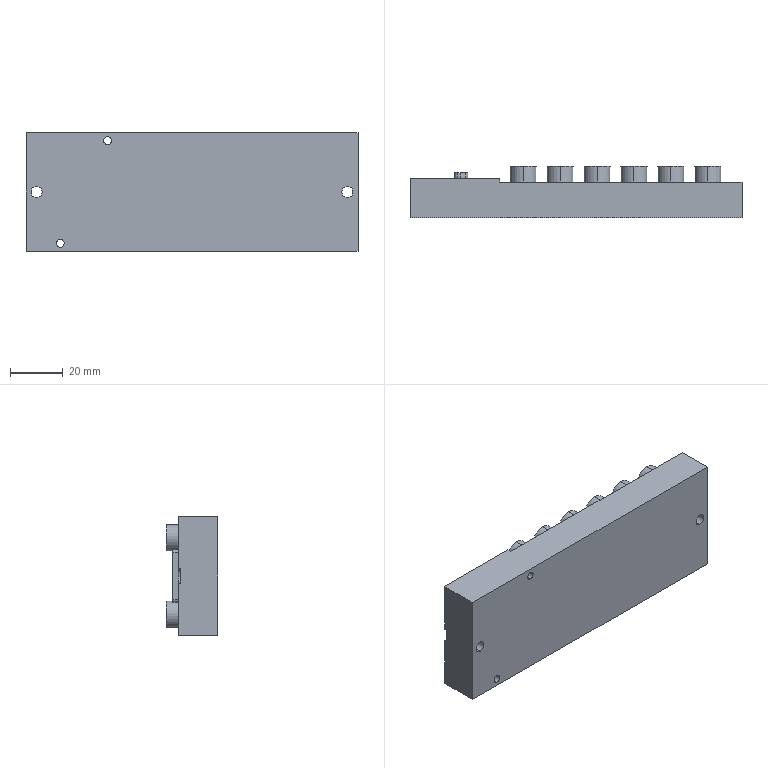Part | STEP file | PRODUCT_NAME_42 | 1 solid | 179 faces | box 126 x 19.5 x 45 mm | volume 83234 mm3 | cylinder 86 | plane 57 | cone 36 | commonest cylinder face diameters 8 x24 9 x24 10 x24 3 x6 4.2 x4 2 x2